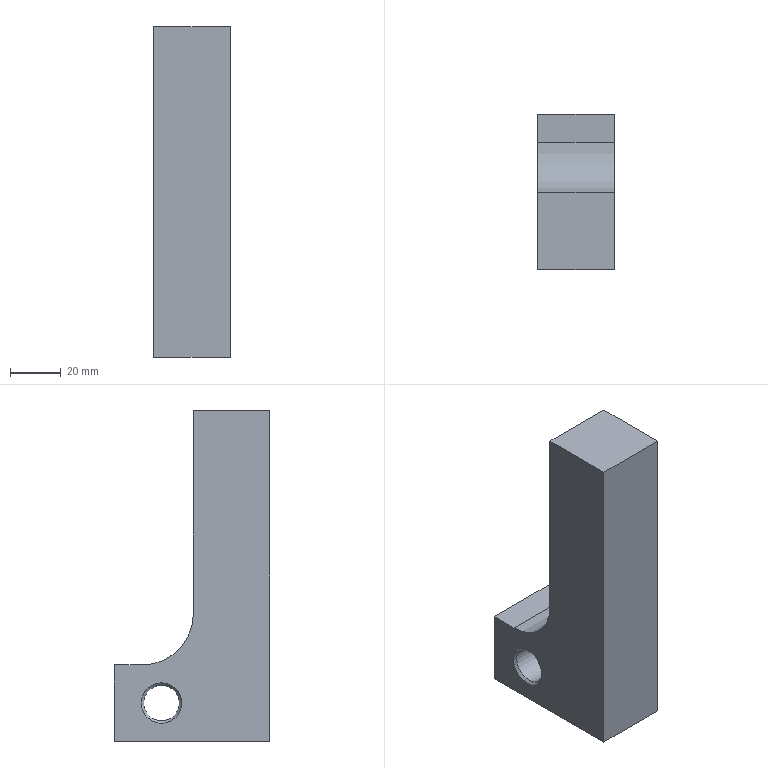Part | STEP file | Tube feed_id550_x_t | 1 solid | 12 faces | box 30 x 61 x 130 mm | volume 142811 mm3 | plane 8 | cylinder 2 | cone 2 | commonest cylinder face diameters 14 x1 40 x1
STEP:
#1=CARTESIAN_POINT('',(0.,0.,0.));
#2=DIRECTION('',(0.,0.,1.));
#3=DIRECTION('',(1.,0.,0.));
#4=AXIS2_PLACEMENT_3D('',#1,#2,#3);
#5=CARTESIAN_POINT('',(176.,541.936,-131.5));
#6=VERTEX_POINT('',#5);
#7=CARTESIAN_POINT('',(176.,552.936,-131.5));
#8=VERTEX_POINT('',#7);
#9=CARTESIAN_POINT('',(176.,521.936,-131.5));
#10=DIRECTION('',(0.,1.,0.));
#11=VECTOR('',#10,1.);
#12=LINE('',#9,#11);
#13=CARTESIAN_POINT('',(176.,521.936,-131.5));
#14=DIRECTION('',(0.,0.,1.));
#15=DIRECTION('',(1.,0.,0.));
#16=AXIS2_PLACEMENT_3D('',#13,#14,#15);
#17=PLANE('',#16);
#18=CARTESIAN_POINT('',(0.,0.));
#19=DIRECTION('',(0.,1.));
#20=VECTOR('',#19,1.);
#21=LINE('',#18,#20);
#22=(GEOMETRIC_REPRESENTATION_CONTEXT(2)PARAMETRIC_REPRESENTATION_CONTEXT()REPRESENTATION_CONTEXT('',''));
#23=DEFINITIONAL_REPRESENTATION('',(#21),#22);
#24=PCURVE('',#17,#23);
#25=CARTESIAN_POINT('',(176.,521.936,-131.5));
#26=DIRECTION('',(1.,0.,0.));
#27=DIRECTION('',(0.,0.,-1.));
#28=AXIS2_PLACEMENT_3D('',#25,#26,#27);
#29=PLANE('',#28);
#30=CARTESIAN_POINT('',(0.,0.));
#31=DIRECTION('',(0.,1.));
#32=VECTOR('',#31,1.);
#33=LINE('',#30,#32);
#34=(GEOMETRIC_REPRESENTATION_CONTEXT(2)PARAMETRIC_REPRESENTATION_CONTEXT()REPRESENTATION_CONTEXT('',''));
#35=DEFINITIONAL_REPRESENTATION('',(#33),#34);
#36=PCURVE('',#29,#35);
#37=SURFACE_CURVE('',#12,(#24,#36),.PCURVE_S1.);
#38=EDGE_CURVE('',#6,#8,#37,.T.);
#39=ORIENTED_EDGE('',*,*,#38,.F.);
#40=CARTESIAN_POINT('',(206.,541.936,-131.5));
#41=VERTEX_POINT('',#40);
#42=CARTESIAN_POINT('',(206.,541.936,-131.5));
#43=DIRECTION('',(1.,0.,0.));
#44=VECTOR('',#43,1.);
#45=LINE('',#42,#44);
#46=CARTESIAN_POINT('',(30.,20.));
#47=DIRECTION('',(1.,0.));
#48=VECTOR('',#47,1.);
#49=LINE('',#46,#48);
#50=(GEOMETRIC_REPRESENTATION_CONTEXT(2)PARAMETRIC_REPRESENTATION_CONTEXT()REPRESENTATION_CONTEXT('',''));
#51=DEFINITIONAL_REPRESENTATION('',(#49),#50);
#52=PCURVE('',#17,#51);
#53=CARTESIAN_POINT('',(176.,541.936,-111.5));
#54=DIRECTION('',(1.,0.,0.));
#55=DIRECTION('',(0.,0.,-1.));
#56=AXIS2_PLACEMENT_3D('',#53,#54,#55);
#57=CYLINDRICAL_SURFACE('',#56,20.);
#58=CARTESIAN_POINT('',(6.283,30.));
#59=DIRECTION('',(0.,1.));
#60=VECTOR('',#59,1.);
#61=LINE('',#58,#60);
#62=(GEOMETRIC_REPRESENTATION_CONTEXT(2)PARAMETRIC_REPRESENTATION_CONTEXT()REPRESENTATION_CONTEXT('',''));
#63=DEFINITIONAL_REPRESENTATION('',(#61),#62);
#64=PCURVE('',#57,#63);
#65=SURFACE_CURVE('',#45,(#52,#64),.PCURVE_S1.);
#66=EDGE_CURVE('',#6,#41,#65,.T.);
#67=ORIENTED_EDGE('',*,*,#66,.T.);
#68=CARTESIAN_POINT('',(206.,552.936,-131.5));
#69=VERTEX_POINT('',#68);
#70=CARTESIAN_POINT('',(206.,521.936,-131.5));
#71=DIRECTION('',(0.,1.,0.));
#72=VECTOR('',#71,1.);
#73=LINE('',#70,#72);
#74=CARTESIAN_POINT('',(30.,0.));
#75=DIRECTION('',(0.,1.));
#76=VECTOR('',#75,1.);
#77=LINE('',#74,#76);
#78=(GEOMETRIC_REPRESENTATION_CONTEXT(2)PARAMETRIC_REPRESENTATION_CONTEXT()REPRESENTATION_CONTEXT('',''));
#79=DEFINITIONAL_REPRESENTATION('',(#77),#78);
#80=PCURVE('',#17,#79);
#81=CARTESIAN_POINT('',(206.,521.936,-131.5));
#82=DIRECTION('',(1.,0.,0.));
#83=DIRECTION('',(0.,0.,-1.));
#84=AXIS2_PLACEMENT_3D('',#81,#82,#83);
#85=PLANE('',#84);
#86=CARTESIAN_POINT('',(0.,0.));
#87=DIRECTION('',(0.,1.));
#88=VECTOR('',#87,1.);
#89=LINE('',#86,#88);
#90=(GEOMETRIC_REPRESENTATION_CONTEXT(2)PARAMETRIC_REPRESENTATION_CONTEXT()REPRESENTATION_CONTEXT('',''));
#91=DEFINITIONAL_REPRESENTATION('',(#89),#90);
#92=PCURVE('',#85,#91);
#93=SURFACE_CURVE('',#73,(#80,#92),.PCURVE_S1.);
#94=EDGE_CURVE('',#41,#69,#93,.T.);
#95=ORIENTED_EDGE('',*,*,#94,.T.);
#96=CARTESIAN_POINT('',(176.,552.936,-131.5));
#97=DIRECTION('',(1.,0.,0.));
#98=VECTOR('',#97,1.);
#99=LINE('',#96,#98);
#100=CARTESIAN_POINT('',(0.,31.));
#101=DIRECTION('',(1.,0.));
#102=VECTOR('',#101,1.);
#103=LINE('',#100,#102);
#104=(GEOMETRIC_REPRESENTATION_CONTEXT(2)PARAMETRIC_REPRESENTATION_CONTEXT()REPRESENTATION_CONTEXT('',''));
#105=DEFINITIONAL_REPRESENTATION('',(#103),#104);
#106=PCURVE('',#17,#105);
#107=CARTESIAN_POINT('',(176.,552.936,-131.5));
#108=DIRECTION('',(0.,1.,0.));
#109=DIRECTION('',(0.,0.,1.));
#110=AXIS2_PLACEMENT_3D('',#107,#108,#109);
#111=PLANE('',#110);
#112=CARTESIAN_POINT('',(0.,0.));
#113=DIRECTION('',(0.,1.));
#114=VECTOR('',#113,1.);
#115=LINE('',#112,#114);
#116=(GEOMETRIC_REPRESENTATION_CONTEXT(2)PARAMETRIC_REPRESENTATION_CONTEXT()REPRESENTATION_CONTEXT('',''));
#117=DEFINITIONAL_REPRESENTATION('',(#115),#116);
#118=PCURVE('',#111,#117);
#119=SURFACE_CURVE('',#99,(#106,#118),.PCURVE_S1.);
#120=EDGE_CURVE('',#8,#69,#119,.T.);
#121=ORIENTED_EDGE('',*,*,#120,.F.);
#122=EDGE_LOOP('',(#39,#67,#95,#121));
#123=FACE_BOUND('',#122,.T.);
#124=ADVANCED_FACE('',(#123),#17,.T.);
#125=CARTESIAN_POINT('',(176.,534.436,-154.5));
#126=VERTEX_POINT('',#125);
#127=CARTESIAN_POINT('',(176.,534.436,-146.5));
#128=DIRECTION('',(1.,0.,0.));
#129=DIRECTION('',(0.,0.,-1.));
#130=AXIS2_PLACEMENT_3D('',#127,#128,#129);
#131=CIRCLE('',#130,8.);
#132=CARTESIAN_POINT('',(15.,12.5));
#133=DIRECTION('',(1.,0.));
#134=AXIS2_PLACEMENT_2D('',#132,#133);
#135=CIRCLE('',#134,8.);
#136=(GEOMETRIC_REPRESENTATION_CONTEXT(2)PARAMETRIC_REPRESENTATION_CONTEXT()REPRESENTATION_CONTEXT('',''));
#137=DEFINITIONAL_REPRESENTATION('',(#135),#136);
#138=PCURVE('',#29,#137);
#139=CARTESIAN_POINT('',(176.,534.436,-146.5));
#140=DIRECTION('',(-1.,0.,0.));
#141=DIRECTION('',(0.,0.,1.));
#142=AXIS2_PLACEMENT_3D('',#139,#140,#141);
#143=CONICAL_SURFACE('',#142,8.,0.7854);
#144=CARTESIAN_POINT('',(9.425,0.));
#145=DIRECTION('',(-1.,0.));
#146=VECTOR('',#145,1.);
#147=LINE('',#144,#146);
#148=(GEOMETRIC_REPRESENTATION_CONTEXT(2)PARAMETRIC_REPRESENTATION_CONTEXT()REPRESENTATION_CONTEXT('',''));
#149=DEFINITIONAL_REPRESENTATION('',(#147),#148);
#150=PCURVE('',#143,#149);
#151=SURFACE_CURVE('',#131,(#138,#150),.PCURVE_S1.);
#152=EDGE_CURVE('',#126,#126,#151,.T.);
#153=ORIENTED_EDGE('',*,*,#152,.T.);
#154=EDGE_LOOP('',(#153));
#155=FACE_BOUND('',#154,.T.);
#156=CARTESIAN_POINT('',(176.,521.936,-31.5));
#157=VERTEX_POINT('',#156);
#158=CARTESIAN_POINT('',(176.,521.936,-111.5));
#159=VERTEX_POINT('',#158);
#160=CARTESIAN_POINT('',(176.,521.936,-31.5));
#161=DIRECTION('',(0.,0.,-1.));
#162=VECTOR('',#161,1.);
#163=LINE('',#160,#162);
#164=CARTESIAN_POINT('',(-100.,0.));
#165=DIRECTION('',(1.,0.));
#166=VECTOR('',#165,1.);
#167=LINE('',#164,#166);
#168=(GEOMETRIC_REPRESENTATION_CONTEXT(2)PARAMETRIC_REPRESENTATION_CONTEXT()REPRESENTATION_CONTEXT('',''));
#169=DEFINITIONAL_REPRESENTATION('',(#167),#168);
#170=PCURVE('',#29,#169);
#171=CARTESIAN_POINT('',(0.,521.936,0.));
#172=DIRECTION('',(0.,-1.,0.));
#173=DIRECTION('',(0.,0.,-1.));
#174=AXIS2_PLACEMENT_3D('',#171,#172,#173);
#175=PLANE('',#174);
#176=CARTESIAN_POINT('',(31.5,176.));
#177=DIRECTION('',(1.,0.));
#178=VECTOR('',#177,1.);
#179=LINE('',#176,#178);
#180=(GEOMETRIC_REPRESENTATION_CONTEXT(2)PARAMETRIC_REPRESENTATION_CONTEXT()REPRESENTATION_CONTEXT('',''));
#181=DEFINITIONAL_REPRESENTATION('',(#179),#180);
#182=PCURVE('',#175,#181);
#183=SURFACE_CURVE('',#163,(#170,#182),.PCURVE_S1.);
#184=EDGE_CURVE('',#157,#159,#183,.T.);
#185=ORIENTED_EDGE('',*,*,#184,.T.);
#186=CARTESIAN_POINT('',(176.,541.936,-111.5));
#187=DIRECTION('',(1.,0.,0.));
#188=DIRECTION('',(0.,0.,-1.));
#189=AXIS2_PLACEMENT_3D('',#186,#187,#188);
#190=CIRCLE('',#189,20.);
#191=CARTESIAN_POINT('',(-20.,20.));
#192=DIRECTION('',(1.,0.));
#193=AXIS2_PLACEMENT_2D('',#191,#192);
#194=CIRCLE('',#193,20.);
#195=(GEOMETRIC_REPRESENTATION_CONTEXT(2)PARAMETRIC_REPRESENTATION_CONTEXT()REPRESENTATION_CONTEXT('',''));
#196=DEFINITIONAL_REPRESENTATION('',(#194),#195);
#197=PCURVE('',#29,#196);
#198=CARTESIAN_POINT('',(0.,0.));
#199=DIRECTION('',(1.,0.));
#200=VECTOR('',#199,1.);
#201=LINE('',#198,#200);
#202=(GEOMETRIC_REPRESENTATION_CONTEXT(2)PARAMETRIC_REPRESENTATION_CONTEXT()REPRESENTATION_CONTEXT('',''));
#203=DEFINITIONAL_REPRESENTATION('',(#201),#202);
#204=PCURVE('',#57,#203);
#205=SURFACE_CURVE('',#190,(#197,#204),.PCURVE_S1.);
#206=EDGE_CURVE('',#159,#6,#205,.T.);
#207=ORIENTED_EDGE('',*,*,#206,.T.);
#208=ORIENTED_EDGE('',*,*,#38,.T.);
#209=CARTESIAN_POINT('',(176.,552.936,-161.5));
#210=VERTEX_POINT('',#209);
#211=CARTESIAN_POINT('',(176.,552.936,-131.5));
#212=DIRECTION('',(0.,0.,-1.));
#213=VECTOR('',#212,1.);
#214=LINE('',#211,#213);
#215=CARTESIAN_POINT('',(0.,31.));
#216=DIRECTION('',(1.,0.));
#217=VECTOR('',#216,1.);
#218=LINE('',#215,#217);
#219=(GEOMETRIC_REPRESENTATION_CONTEXT(2)PARAMETRIC_REPRESENTATION_CONTEXT()REPRESENTATION_CONTEXT('',''));
#220=DEFINITIONAL_REPRESENTATION('',(#218),#219);
#221=PCURVE('',#29,#220);
#222=CARTESIAN_POINT('',(0.,0.));
#223=DIRECTION('',(-1.,0.));
#224=VECTOR('',#223,1.);
#225=LINE('',#222,#224);
#226=(GEOMETRIC_REPRESENTATION_CONTEXT(2)PARAMETRIC_REPRESENTATION_CONTEXT()REPRESENTATION_CONTEXT('',''));
#227=DEFINITIONAL_REPRESENTATION('',(#225),#226);
#228=PCURVE('',#111,#227);
#229=SURFACE_CURVE('',#214,(#221,#228),.PCURVE_S1.);
#230=EDGE_CURVE('',#8,#210,#229,.T.);
#231=ORIENTED_EDGE('',*,*,#230,.T.);
#232=CARTESIAN_POINT('',(176.,491.936,-161.5));
#233=VERTEX_POINT('',#232);
#234=CARTESIAN_POINT('',(176.,521.936,-161.5));
#235=DIRECTION('',(0.,-1.,0.));
#236=VECTOR('',#235,1.);
#237=LINE('',#234,#236);
#238=CARTESIAN_POINT('',(30.,0.));
#239=DIRECTION('',(0.,-1.));
#240=VECTOR('',#239,1.);
#241=LINE('',#238,#240);
#242=(GEOMETRIC_REPRESENTATION_CONTEXT(2)PARAMETRIC_REPRESENTATION_CONTEXT()REPRESENTATION_CONTEXT('',''));
#243=DEFINITIONAL_REPRESENTATION('',(#241),#242);
#244=PCURVE('',#29,#243);
#245=CARTESIAN_POINT('',(176.,521.936,-161.5));
#246=DIRECTION('',(0.,0.,1.));
#247=DIRECTION('',(1.,0.,0.));
#248=AXIS2_PLACEMENT_3D('',#245,#246,#247);
#249=PLANE('',#248);
#250=CARTESIAN_POINT('',(0.,0.));
#251=DIRECTION('',(0.,-1.));
#252=VECTOR('',#251,1.);
#253=LINE('',#250,#252);
#254=(GEOMETRIC_REPRESENTATION_CONTEXT(2)PARAMETRIC_REPRESENTATION_CONTEXT()REPRESENTATION_CONTEXT('',''));
#255=DEFINITIONAL_REPRESENTATION('',(#253),#254);
#256=PCURVE('',#249,#255);
#257=SURFACE_CURVE('',#237,(#244,#256),.PCURVE_S1.);
#258=EDGE_CURVE('',#210,#233,#257,.T.);
#259=ORIENTED_EDGE('',*,*,#258,.T.);
#260=CARTESIAN_POINT('',(176.,491.936,-31.5));
#261=VERTEX_POINT('',#260);
#262=CARTESIAN_POINT('',(176.,491.936,-31.5));
#263=DIRECTION('',(0.,0.,-1.));
#264=VECTOR('',#263,1.);
#265=LINE('',#262,#264);
#266=CARTESIAN_POINT('',(-100.,-30.));
#267=DIRECTION('',(1.,0.));
#268=VECTOR('',#267,1.);
#269=LINE('',#266,#268);
#270=(GEOMETRIC_REPRESENTATION_CONTEXT(2)PARAMETRIC_REPRESENTATION_CONTEXT()REPRESENTATION_CONTEXT('',''));
#271=DEFINITIONAL_REPRESENTATION('',(#269),#270);
#272=PCURVE('',#29,#271);
#273=CARTESIAN_POINT('',(0.,491.936,0.));
#274=DIRECTION('',(0.,-1.,0.));
#275=DIRECTION('',(0.,0.,-1.));
#276=AXIS2_PLACEMENT_3D('',#273,#274,#275);
#277=PLANE('',#276);
#278=CARTESIAN_POINT('',(31.5,176.));
#279=DIRECTION('',(1.,0.));
#280=VECTOR('',#279,1.);
#281=LINE('',#278,#280);
#282=(GEOMETRIC_REPRESENTATION_CONTEXT(2)PARAMETRIC_REPRESENTATION_CONTEXT()REPRESENTATION_CONTEXT('',''));
#283=DEFINITIONAL_REPRESENTATION('',(#281),#282);
#284=PCURVE('',#277,#283);
#285=SURFACE_CURVE('',#265,(#272,#284),.PCURVE_S1.);
#286=EDGE_CURVE('',#261,#233,#285,.T.);
#287=ORIENTED_EDGE('',*,*,#286,.F.);
#288=CARTESIAN_POINT('',(176.,521.936,-31.5));
#289=DIRECTION('',(0.,-1.,0.));
#290=VECTOR('',#289,1.);
#291=LINE('',#288,#290);
#292=CARTESIAN_POINT('',(-100.,0.));
#293=DIRECTION('',(0.,-1.));
#294=VECTOR('',#293,1.);
#295=LINE('',#292,#294);
#296=(GEOMETRIC_REPRESENTATION_CONTEXT(2)PARAMETRIC_REPRESENTATION_CONTEXT()REPRESENTATION_CONTEXT('',''));
#297=DEFINITIONAL_REPRESENTATION('',(#295),#296);
#298=PCURVE('',#29,#297);
#299=CARTESIAN_POINT('',(206.,521.936,-31.5));
#300=DIRECTION('',(0.,0.,1.));
#301=DIRECTION('',(1.,0.,0.));
#302=AXIS2_PLACEMENT_3D('',#299,#300,#301);
#303=PLANE('',#302);
#304=CARTESIAN_POINT('',(-30.,0.));
#305=DIRECTION('',(0.,-1.));
#306=VECTOR('',#305,1.);
#307=LINE('',#304,#306);
#308=(GEOMETRIC_REPRESENTATION_CONTEXT(2)PARAMETRIC_REPRESENTATION_CONTEXT()REPRESENTATION_CONTEXT('',''));
#309=DEFINITIONAL_REPRESENTATION('',(#307),#308);
#310=PCURVE('',#303,#309);
#311=SURFACE_CURVE('',#291,(#298,#310),.PCURVE_S1.);
#312=EDGE_CURVE('',#157,#261,#311,.T.);
#313=ORIENTED_EDGE('',*,*,#312,.F.);
#314=EDGE_LOOP('',(#185,#207,#208,#231,#259,#287,#313));
#315=FACE_BOUND('',#314,.T.);
#316=ADVANCED_FACE('',(#155,#315),#29,.F.);
#317=ORIENTED_EDGE('',*,*,#258,.F.);
#318=CARTESIAN_POINT('',(206.,552.936,-161.5));
#319=VERTEX_POINT('',#318);
#320=CARTESIAN_POINT('',(176.,552.936,-161.5));
#321=DIRECTION('',(1.,0.,0.));
#322=VECTOR('',#321,1.);
#323=LINE('',#320,#322);
#324=CARTESIAN_POINT('',(0.,31.));
#325=DIRECTION('',(1.,0.));
#326=VECTOR('',#325,1.);
#327=LINE('',#324,#326);
#328=(GEOMETRIC_REPRESENTATION_CONTEXT(2)PARAMETRIC_REPRESENTATION_CONTEXT()REPRESENTATION_CONTEXT('',''));
#329=DEFINITIONAL_REPRESENTATION('',(#327),#328);
#330=PCURVE('',#249,#329);
#331=CARTESIAN_POINT('',(-30.,0.));
#332=DIRECTION('',(0.,1.));
#333=VECTOR('',#332,1.);
#334=LINE('',#331,#333);
#335=(GEOMETRIC_REPRESENTATION_CONTEXT(2)PARAMETRIC_REPRESENTATION_CONTEXT()REPRESENTATION_CONTEXT('',''));
#336=DEFINITIONAL_REPRESENTATION('',(#334),#335);
#337=PCURVE('',#111,#336);
#338=SURFACE_CURVE('',#323,(#330,#337),.PCURVE_S1.);
#339=EDGE_CURVE('',#210,#319,#338,.T.);
#340=ORIENTED_EDGE('',*,*,#339,.T.);
#341=CARTESIAN_POINT('',(206.,491.936,-161.5));
#342=VERTEX_POINT('',#341);
#343=CARTESIAN_POINT('',(206.,521.936,-161.5));
#344=DIRECTION('',(0.,-1.,0.));
#345=VECTOR('',#344,1.);
#346=LINE('',#343,#345);
#347=CARTESIAN_POINT('',(30.,0.));
#348=DIRECTION('',(0.,-1.));
#349=VECTOR('',#348,1.);
#350=LINE('',#347,#349);
#351=(GEOMETRIC_REPRESENTATION_CONTEXT(2)PARAMETRIC_REPRESENTATION_CONTEXT()REPRESENTATION_CONTEXT('',''));
#352=DEFINITIONAL_REPRESENTATION('',(#350),#351);
#353=PCURVE('',#249,#352);
#354=CARTESIAN_POINT('',(30.,0.));
#355=DIRECTION('',(0.,-1.));
#356=VECTOR('',#355,1.);
#357=LINE('',#354,#356);
#358=(GEOMETRIC_REPRESENTATION_CONTEXT(2)PARAMETRIC_REPRESENTATION_CONTEXT()REPRESENTATION_CONTEXT('',''));
#359=DEFINITIONAL_REPRESENTATION('',(#357),#358);
#360=PCURVE('',#85,#359);
#361=SURFACE_CURVE('',#346,(#353,#360),.PCURVE_S1.);
#362=EDGE_CURVE('',#319,#342,#361,.T.);
#363=ORIENTED_EDGE('',*,*,#362,.T.);
#364=CARTESIAN_POINT('',(176.,491.936,-161.5));
#365=DIRECTION('',(1.,0.,0.));
#366=VECTOR('',#365,1.);
#367=LINE('',#364,#366);
#368=CARTESIAN_POINT('',(0.,-30.));
#369=DIRECTION('',(1.,0.));
#370=VECTOR('',#369,1.);
#371=LINE('',#368,#370);
#372=(GEOMETRIC_REPRESENTATION_CONTEXT(2)PARAMETRIC_REPRESENTATION_CONTEXT()REPRESENTATION_CONTEXT('',''));
#373=DEFINITIONAL_REPRESENTATION('',(#371),#372);
#374=PCURVE('',#249,#373);
#375=CARTESIAN_POINT('',(161.5,176.));
#376=DIRECTION('',(0.,1.));
#377=VECTOR('',#376,1.);
#378=LINE('',#375,#377);
#379=(GEOMETRIC_REPRESENTATION_CONTEXT(2)PARAMETRIC_REPRESENTATION_CONTEXT()REPRESENTATION_CONTEXT('',''));
#380=DEFINITIONAL_REPRESENTATION('',(#378),#379);
#381=PCURVE('',#277,#380);
#382=SURFACE_CURVE('',#367,(#374,#381),.PCURVE_S1.);
#383=EDGE_CURVE('',#233,#342,#382,.T.);
#384=ORIENTED_EDGE('',*,*,#383,.F.);
#385=EDGE_LOOP('',(#317,#340,#363,#384));
#386=FACE_BOUND('',#385,.T.);
#387=ADVANCED_FACE('',(#386),#249,.F.);
#388=CARTESIAN_POINT('',(206.,534.436,-154.5));
#389=VERTEX_POINT('',#388);
#390=CARTESIAN_POINT('',(206.,534.436,-146.5));
#391=DIRECTION('',(-1.,0.,0.));
#392=DIRECTION('',(0.,0.,-1.));
#393=AXIS2_PLACEMENT_3D('',#390,#391,#392);
#394=CIRCLE('',#393,8.);
#395=CARTESIAN_POINT('',(23.,12.5));
#396=CARTESIAN_POINT('',(23.,-1.356));
#397=CARTESIAN_POINT('',(11.,5.572));
#398=CARTESIAN_POINT('',(-1.,12.5));
#399=CARTESIAN_POINT('',(11.,19.428));
#400=CARTESIAN_POINT('',(23.,26.356));
#401=CARTESIAN_POINT('',(23.,12.5));
#402=(BOUNDED_CURVE()B_SPLINE_CURVE(2,(#395,#396,#397,#398,#399,#400,#401),.UNSPECIFIED.,.T.,.F.)B_SPLINE_CURVE_WITH_KNOTS((1,2,2,2,2,1),(-2.094,0.,2.094,4.189,6.283,8.378),.UNSPECIFIED.)CURVE()GEOMETRIC_REPRESENTATION_ITEM()RATIONAL_B_SPLINE_CURVE((1.,0.5,1.,0.5,1.,0.5,1.))REPRESENTATION_ITEM(''));
#403=(GEOMETRIC_REPRESENTATION_CONTEXT(2)PARAMETRIC_REPRESENTATION_CONTEXT()REPRESENTATION_CONTEXT('',''));
#404=DEFINITIONAL_REPRESENTATION('',(#402),#403);
#405=PCURVE('',#85,#404);
#406=CARTESIAN_POINT('',(206.,534.436,-146.5));
#407=DIRECTION('',(1.,0.,0.));
#408=DIRECTION('',(0.,0.,-1.));
#409=AXIS2_PLACEMENT_3D('',#406,#407,#408);
#410=CONICAL_SURFACE('',#409,8.,0.7854);
#411=CARTESIAN_POINT('',(6.283,0.));
#412=DIRECTION('',(-1.,0.));
#413=VECTOR('',#412,1.);
#414=LINE('',#411,#413);
#415=(GEOMETRIC_REPRESENTATION_CONTEXT(2)PARAMETRIC_REPRESENTATION_CONTEXT()REPRESENTATION_CONTEXT('',''));
#416=DEFINITIONAL_REPRESENTATION('',(#414),#415);
#417=PCURVE('',#410,#416);
#418=SURFACE_CURVE('',#394,(#405,#417),.PCURVE_S1.);
#419=EDGE_CURVE('',#389,#389,#418,.T.);
#420=ORIENTED_EDGE('',*,*,#419,.T.);
#421=EDGE_LOOP('',(#420));
#422=FACE_BOUND('',#421,.T.);
#423=ORIENTED_EDGE('',*,*,#94,.F.);
#424=CARTESIAN_POINT('',(206.,521.936,-111.5));
#425=VERTEX_POINT('',#424);
#426=CARTESIAN_POINT('',(206.,541.936,-111.5));
#427=DIRECTION('',(-1.,0.,0.));
#428=DIRECTION('',(0.,0.,-1.));
#429=AXIS2_PLACEMENT_3D('',#426,#427,#428);
#430=CIRCLE('',#429,20.);
#431=CARTESIAN_POINT('',(0.,20.));
#432=CARTESIAN_POINT('',(0.,-14.641));
#433=CARTESIAN_POINT('',(-30.,2.679));
#434=CARTESIAN_POINT('',(-60.,20.));
#435=CARTESIAN_POINT('',(-30.,37.321));
#436=CARTESIAN_POINT('',(0.,54.641));
#437=CARTESIAN_POINT('',(0.,20.));
#438=(BOUNDED_CURVE()B_SPLINE_CURVE(2,(#431,#432,#433,#434,#435,#436,#437),.UNSPECIFIED.,.T.,.F.)B_SPLINE_CURVE_WITH_KNOTS((1,2,2,2,2,1),(-2.094,0.,2.094,4.189,6.283,8.378),.UNSPECIFIED.)CURVE()GEOMETRIC_REPRESENTATION_ITEM()RATIONAL_B_SPLINE_CURVE((1.,0.5,1.,0.5,1.,0.5,1.))REPRESENTATION_ITEM(''));
#439=(GEOMETRIC_REPRESENTATION_CONTEXT(2)PARAMETRIC_REPRESENTATION_CONTEXT()REPRESENTATION_CONTEXT('',''));
#440=DEFINITIONAL_REPRESENTATION('',(#438),#439);
#441=PCURVE('',#85,#440);
#442=CARTESIAN_POINT('',(6.283,30.));
#443=DIRECTION('',(-1.,0.));
#444=VECTOR('',#443,1.);
#445=LINE('',#442,#444);
#446=(GEOMETRIC_REPRESENTATION_CONTEXT(2)PARAMETRIC_REPRESENTATION_CONTEXT()REPRESENTATION_CONTEXT('',''));
#447=DEFINITIONAL_REPRESENTATION('',(#445),#446);
#448=PCURVE('',#57,#447);
#449=SURFACE_CURVE('',#430,(#441,#448),.PCURVE_S1.);
#450=EDGE_CURVE('',#41,#425,#449,.T.);
#451=ORIENTED_EDGE('',*,*,#450,.T.);
#452=CARTESIAN_POINT('',(206.,521.936,-31.5));
#453=VERTEX_POINT('',#452);
#454=CARTESIAN_POINT('',(206.,521.936,-161.5));
#455=DIRECTION('',(0.,0.,1.));
#456=VECTOR('',#455,1.);
#457=LINE('',#454,#456);
#458=CARTESIAN_POINT('',(30.,0.));
#459=DIRECTION('',(-1.,0.));
#460=VECTOR('',#459,1.);
#461=LINE('',#458,#460);
#462=(GEOMETRIC_REPRESENTATION_CONTEXT(2)PARAMETRIC_REPRESENTATION_CONTEXT()REPRESENTATION_CONTEXT('',''));
#463=DEFINITIONAL_REPRESENTATION('',(#461),#462);
#464=PCURVE('',#85,#463);
#465=CARTESIAN_POINT('',(161.5,206.));
#466=DIRECTION('',(-1.,0.));
#467=VECTOR('',#466,1.);
#468=LINE('',#465,#467);
#469=(GEOMETRIC_REPRESENTATION_CONTEXT(2)PARAMETRIC_REPRESENTATION_CONTEXT()REPRESENTATION_CONTEXT('',''));
#470=DEFINITIONAL_REPRESENTATION('',(#468),#469);
#471=PCURVE('',#175,#470);
#472=SURFACE_CURVE('',#457,(#464,#471),.PCURVE_S1.);
#473=EDGE_CURVE('',#425,#453,#472,.T.);
#474=ORIENTED_EDGE('',*,*,#473,.T.);
#475=CARTESIAN_POINT('',(206.,491.936,-31.5));
#476=VERTEX_POINT('',#475);
#477=CARTESIAN_POINT('',(206.,521.936,-31.5));
#478=DIRECTION('',(0.,-1.,0.));
#479=VECTOR('',#478,1.);
#480=LINE('',#477,#479);
#481=CARTESIAN_POINT('',(-100.,0.));
#482=DIRECTION('',(0.,-1.));
#483=VECTOR('',#482,1.);
#484=LINE('',#481,#483);
#485=(GEOMETRIC_REPRESENTATION_CONTEXT(2)PARAMETRIC_REPRESENTATION_CONTEXT()REPRESENTATION_CONTEXT('',''));
#486=DEFINITIONAL_REPRESENTATION('',(#484),#485);
#487=PCURVE('',#85,#486);
#488=CARTESIAN_POINT('',(0.,0.));
#489=DIRECTION('',(0.,-1.));
#490=VECTOR('',#489,1.);
#491=LINE('',#488,#490);
#492=(GEOMETRIC_REPRESENTATION_CONTEXT(2)PARAMETRIC_REPRESENTATION_CONTEXT()REPRESENTATION_CONTEXT('',''));
#493=DEFINITIONAL_REPRESENTATION('',(#491),#492);
#494=PCURVE('',#303,#493);
#495=SURFACE_CURVE('',#480,(#487,#494),.PCURVE_S1.);
#496=EDGE_CURVE('',#453,#476,#495,.T.);
#497=ORIENTED_EDGE('',*,*,#496,.T.);
#498=CARTESIAN_POINT('',(206.,491.936,-161.5));
#499=DIRECTION('',(0.,0.,1.));
#500=VECTOR('',#499,1.);
#501=LINE('',#498,#500);
#502=CARTESIAN_POINT('',(30.,-30.));
#503=DIRECTION('',(-1.,0.));
#504=VECTOR('',#503,1.);
#505=LINE('',#502,#504);
#506=(GEOMETRIC_REPRESENTATION_CONTEXT(2)PARAMETRIC_REPRESENTATION_CONTEXT()REPRESENTATION_CONTEXT('',''));
#507=DEFINITIONAL_REPRESENTATION('',(#505),#506);
#508=PCURVE('',#85,#507);
#509=CARTESIAN_POINT('',(161.5,206.));
#510=DIRECTION('',(-1.,0.));
#511=VECTOR('',#510,1.);
#512=LINE('',#509,#511);
#513=(GEOMETRIC_REPRESENTATION_CONTEXT(2)PARAMETRIC_REPRESENTATION_CONTEXT()REPRESENTATION_CONTEXT('',''));
#514=DEFINITIONAL_REPRESENTATION('',(#512),#513);
#515=PCURVE('',#277,#514);
#516=SURFACE_CURVE('',#501,(#508,#515),.PCURVE_S1.);
#517=EDGE_CURVE('',#342,#476,#516,.T.);
#518=ORIENTED_EDGE('',*,*,#517,.F.);
#519=ORIENTED_EDGE('',*,*,#362,.F.);
#520=CARTESIAN_POINT('',(206.,552.936,-131.5));
#521=DIRECTION('',(0.,0.,-1.));
#522=VECTOR('',#521,1.);
#523=LINE('',#520,#522);
#524=CARTESIAN_POINT('',(0.,31.));
#525=DIRECTION('',(1.,0.));
#526=VECTOR('',#525,1.);
#527=LINE('',#524,#526);
#528=(GEOMETRIC_REPRESENTATION_CONTEXT(2)PARAMETRIC_REPRESENTATION_CONTEXT()REPRESENTATION_CONTEXT('',''));
#529=DEFINITIONAL_REPRESENTATION('',(#527),#528);
#530=PCURVE('',#85,#529);
#531=CARTESIAN_POINT('',(0.,30.));
#532=DIRECTION('',(-1.,0.));
#533=VECTOR('',#532,1.);
#534=LINE('',#531,#533);
#535=(GEOMETRIC_REPRESENTATION_CONTEXT(2)PARAMETRIC_REPRESENTATION_CONTEXT()REPRESENTATION_CONTEXT('',''));
#536=DEFINITIONAL_REPRESENTATION('',(#534),#535);
#537=PCURVE('',#111,#536);
#538=SURFACE_CURVE('',#523,(#530,#537),.PCURVE_S1.);
#539=EDGE_CURVE('',#69,#319,#538,.T.);
#540=ORIENTED_EDGE('',*,*,#539,.F.);
#541=EDGE_LOOP('',(#423,#451,#474,#497,#518,#519,#540));
#542=FACE_BOUND('',#541,.T.);
#543=ADVANCED_FACE('',(#422,#542),#85,.T.);
#544=ORIENTED_EDGE('',*,*,#339,.F.);
#545=ORIENTED_EDGE('',*,*,#230,.F.);
#546=ORIENTED_EDGE('',*,*,#120,.T.);
#547=ORIENTED_EDGE('',*,*,#539,.T.);
#548=EDGE_LOOP('',(#544,#545,#546,#547));
#549=FACE_BOUND('',#548,.T.);
#550=ADVANCED_FACE('',(#549),#111,.T.);
#551=CARTESIAN_POINT('',(206.,491.936,-31.5));
#552=DIRECTION('',(-1.,0.,0.));
#553=VECTOR('',#552,1.);
#554=LINE('',#551,#553);
#555=CARTESIAN_POINT('',(0.,-30.));
#556=DIRECTION('',(-1.,0.));
#557=VECTOR('',#556,1.);
#558=LINE('',#555,#557);
#559=(GEOMETRIC_REPRESENTATION_CONTEXT(2)PARAMETRIC_REPRESENTATION_CONTEXT()REPRESENTATION_CONTEXT('',''));
#560=DEFINITIONAL_REPRESENTATION('',(#558),#559);
#561=PCURVE('',#303,#560);
#562=CARTESIAN_POINT('',(31.5,206.));
#563=DIRECTION('',(0.,-1.));
#564=VECTOR('',#563,1.);
#565=LINE('',#562,#564);
#566=(GEOMETRIC_REPRESENTATION_CONTEXT(2)PARAMETRIC_REPRESENTATION_CONTEXT()REPRESENTATION_CONTEXT('',''));
#567=DEFINITIONAL_REPRESENTATION('',(#565),#566);
#568=PCURVE('',#277,#567);
#569=SURFACE_CURVE('',#554,(#561,#568),.PCURVE_S1.);
#570=EDGE_CURVE('',#476,#261,#569,.T.);
#571=ORIENTED_EDGE('',*,*,#570,.F.);
#572=ORIENTED_EDGE('',*,*,#496,.F.);
#573=CARTESIAN_POINT('',(206.,521.936,-31.5));
#574=DIRECTION('',(-1.,0.,0.));
#575=VECTOR('',#574,1.);
#576=LINE('',#573,#575);
#577=CARTESIAN_POINT('',(0.,0.));
#578=DIRECTION('',(-1.,0.));
#579=VECTOR('',#578,1.);
#580=LINE('',#577,#579);
#581=(GEOMETRIC_REPRESENTATION_CONTEXT(2)PARAMETRIC_REPRESENTATION_CONTEXT()REPRESENTATION_CONTEXT('',''));
#582=DEFINITIONAL_REPRESENTATION('',(#580),#581);
#583=PCURVE('',#303,#582);
#584=CARTESIAN_POINT('',(31.5,206.));
#585=DIRECTION('',(0.,-1.));
#586=VECTOR('',#585,1.);
#587=LINE('',#584,#586);
#588=(GEOMETRIC_REPRESENTATION_CONTEXT(2)PARAMETRIC_REPRESENTATION_CONTEXT()REPRESENTATION_CONTEXT('',''));
#589=DEFINITIONAL_REPRESENTATION('',(#587),#588);
#590=PCURVE('',#175,#589);
#591=SURFACE_CURVE('',#576,(#583,#590),.PCURVE_S1.);
#592=EDGE_CURVE('',#453,#157,#591,.T.);
#593=ORIENTED_EDGE('',*,*,#592,.T.);
#594=ORIENTED_EDGE('',*,*,#312,.T.);
#595=EDGE_LOOP('',(#571,#572,#593,#594));
#596=FACE_BOUND('',#595,.T.);
#597=ADVANCED_FACE('',(#596),#303,.T.);
#598=ORIENTED_EDGE('',*,*,#473,.F.);
#599=CARTESIAN_POINT('',(176.,521.936,-111.5));
#600=DIRECTION('',(-1.,0.,0.));
#601=VECTOR('',#600,1.);
#602=LINE('',#599,#601);
#603=CARTESIAN_POINT('',(111.5,176.));
#604=DIRECTION('',(0.,-1.));
#605=VECTOR('',#604,1.);
#606=LINE('',#603,#605);
#607=(GEOMETRIC_REPRESENTATION_CONTEXT(2)PARAMETRIC_REPRESENTATION_CONTEXT()REPRESENTATION_CONTEXT('',''));
#608=DEFINITIONAL_REPRESENTATION('',(#606),#607);
#609=PCURVE('',#175,#608);
#610=CARTESIAN_POINT('',(4.712,0.));
#611=DIRECTION('',(0.,-1.));
#612=VECTOR('',#611,1.);
#613=LINE('',#610,#612);
#614=(GEOMETRIC_REPRESENTATION_CONTEXT(2)PARAMETRIC_REPRESENTATION_CONTEXT()REPRESENTATION_CONTEXT('',''));
#615=DEFINITIONAL_REPRESENTATION('',(#613),#614);
#616=PCURVE('',#57,#615);
#617=SURFACE_CURVE('',#602,(#609,#616),.PCURVE_S1.);
#618=EDGE_CURVE('',#425,#159,#617,.T.);
#619=ORIENTED_EDGE('',*,*,#618,.T.);
#620=ORIENTED_EDGE('',*,*,#184,.F.);
#621=ORIENTED_EDGE('',*,*,#592,.F.);
#622=EDGE_LOOP('',(#598,#619,#620,#621));
#623=FACE_BOUND('',#622,.T.);
#624=ADVANCED_FACE('',(#623),#175,.F.);
#625=ORIENTED_EDGE('',*,*,#286,.T.);
#626=ORIENTED_EDGE('',*,*,#383,.T.);
#627=ORIENTED_EDGE('',*,*,#517,.T.);
#628=ORIENTED_EDGE('',*,*,#570,.T.);
#629=EDGE_LOOP('',(#625,#626,#627,#628));
#630=FACE_BOUND('',#629,.T.);
#631=ADVANCED_FACE('',(#630),#277,.T.);
#632=ORIENTED_EDGE('',*,*,#66,.T.);
#633=ORIENTED_EDGE('',*,*,#450,.T.);
#634=ORIENTED_EDGE('',*,*,#618,.T.);
#635=ORIENTED_EDGE('',*,*,#206,.T.);
#636=EDGE_LOOP('',(#632,#633,#634,#635));
#637=FACE_BOUND('',#636,.F.);
#638=ADVANCED_FACE('',(#637),#57,.F.);
#639=CARTESIAN_POINT('',(177.,534.436,-139.5));
#640=VERTEX_POINT('',#639);
#641=CARTESIAN_POINT('',(177.,534.436,-153.5));
#642=VERTEX_POINT('',#641);
#643=CARTESIAN_POINT('',(177.,534.436,-146.5));
#644=DIRECTION('',(-1.,0.,0.));
#645=DIRECTION('',(0.,0.,-1.));
#646=AXIS2_PLACEMENT_3D('',#643,#644,#645);
#647=CIRCLE('',#646,7.);
#648=CARTESIAN_POINT('',(206.,534.436,-146.5));
#649=DIRECTION('',(-1.,0.,0.));
#650=DIRECTION('',(0.,0.,1.));
#651=AXIS2_PLACEMENT_3D('',#648,#649,#650);
#652=CYLINDRICAL_SURFACE('',#651,7.);
#653=CARTESIAN_POINT('',(-3.142,29.));
#654=DIRECTION('',(1.,0.));
#655=VECTOR('',#654,1.);
#656=LINE('',#653,#655);
#657=(GEOMETRIC_REPRESENTATION_CONTEXT(2)PARAMETRIC_REPRESENTATION_CONTEXT()REPRESENTATION_CONTEXT('',''));
#658=DEFINITIONAL_REPRESENTATION('',(#656),#657);
#659=PCURVE('',#652,#658);
#660=CARTESIAN_POINT('',(3.142,-1.));
#661=DIRECTION('',(1.,0.));
#662=VECTOR('',#661,1.);
#663=LINE('',#660,#662);
#664=(GEOMETRIC_REPRESENTATION_CONTEXT(2)PARAMETRIC_REPRESENTATION_CONTEXT()REPRESENTATION_CONTEXT('',''));
#665=DEFINITIONAL_REPRESENTATION('',(#663),#664);
#666=PCURVE('',#143,#665);
#667=SURFACE_CURVE('',#647,(#659,#666),.PCURVE_S1.);
#668=EDGE_CURVE('',#640,#642,#667,.T.);
#669=ORIENTED_EDGE('',*,*,#668,.F.);
#670=CARTESIAN_POINT('',(205.,534.436,-139.5));
#671=VERTEX_POINT('',#670);
#672=CARTESIAN_POINT('',(205.,534.436,-139.5));
#673=CARTESIAN_POINT('',(177.,534.436,-139.5));
#674=B_SPLINE_CURVE_WITH_KNOTS('',1,(#672,#673),.UNSPECIFIED.,.F.,.F.,(2,2),(1.,29.),.PIECEWISE_BEZIER_KNOTS.);
#675=CARTESIAN_POINT('',(0.,0.));
#676=DIRECTION('',(0.,1.));
#677=VECTOR('',#676,1.);
#678=LINE('',#675,#677);
#679=(GEOMETRIC_REPRESENTATION_CONTEXT(2)PARAMETRIC_REPRESENTATION_CONTEXT()REPRESENTATION_CONTEXT('',''));
#680=DEFINITIONAL_REPRESENTATION('',(#678),#679);
#681=PCURVE('',#652,#680);
#682=CARTESIAN_POINT('',(6.283,0.));
#683=DIRECTION('',(0.,1.));
#684=VECTOR('',#683,1.);
#685=LINE('',#682,#684);
#686=(GEOMETRIC_REPRESENTATION_CONTEXT(2)PARAMETRIC_REPRESENTATION_CONTEXT()REPRESENTATION_CONTEXT('',''));
#687=DEFINITIONAL_REPRESENTATION('',(#685),#686);
#688=PCURVE('',#652,#687);
#689=SEAM_CURVE('',#674,(#681,#688),.PCURVE_S1.);
#690=EDGE_CURVE('',#671,#640,#689,.T.);
#691=ORIENTED_EDGE('',*,*,#690,.F.);
#692=CARTESIAN_POINT('',(205.,534.436,-153.5));
#693=VERTEX_POINT('',#692);
#694=CARTESIAN_POINT('',(205.,534.436,-146.5));
#695=DIRECTION('',(1.,0.,0.));
#696=DIRECTION('',(0.,0.,1.));
#697=AXIS2_PLACEMENT_3D('',#694,#695,#696);
#698=CIRCLE('',#697,7.);
#699=CARTESIAN_POINT('',(6.283,1.));
#700=DIRECTION('',(-1.,0.));
#701=VECTOR('',#700,1.);
#702=LINE('',#699,#701);
#703=(GEOMETRIC_REPRESENTATION_CONTEXT(2)PARAMETRIC_REPRESENTATION_CONTEXT()REPRESENTATION_CONTEXT('',''));
#704=DEFINITIONAL_REPRESENTATION('',(#702),#703);
#705=PCURVE('',#652,#704);
#706=CARTESIAN_POINT('',(-3.142,-1.));
#707=DIRECTION('',(1.,0.));
#708=VECTOR('',#707,1.);
#709=LINE('',#706,#708);
#710=(GEOMETRIC_REPRESENTATION_CONTEXT(2)PARAMETRIC_REPRESENTATION_CONTEXT()REPRESENTATION_CONTEXT('',''));
#711=DEFINITIONAL_REPRESENTATION('',(#709),#710);
#712=PCURVE('',#410,#711);
#713=SURFACE_CURVE('',#698,(#705,#712),.PCURVE_S1.);
#714=EDGE_CURVE('',#693,#671,#713,.T.);
#715=ORIENTED_EDGE('',*,*,#714,.F.);
#716=CARTESIAN_POINT('',(205.,534.436,-146.5));
#717=DIRECTION('',(1.,0.,0.));
#718=DIRECTION('',(0.,0.,1.));
#719=AXIS2_PLACEMENT_3D('',#716,#717,#718);
#720=CIRCLE('',#719,7.);
#721=CARTESIAN_POINT('',(6.283,1.));
#722=DIRECTION('',(-1.,0.));
#723=VECTOR('',#722,1.);
#724=LINE('',#721,#723);
#725=(GEOMETRIC_REPRESENTATION_CONTEXT(2)PARAMETRIC_REPRESENTATION_CONTEXT()REPRESENTATION_CONTEXT('',''));
#726=DEFINITIONAL_REPRESENTATION('',(#724),#725);
#727=PCURVE('',#652,#726);
#728=CARTESIAN_POINT('',(3.142,-1.));
#729=DIRECTION('',(1.,0.));
#730=VECTOR('',#729,1.);
#731=LINE('',#728,#730);
#732=(GEOMETRIC_REPRESENTATION_CONTEXT(2)PARAMETRIC_REPRESENTATION_CONTEXT()REPRESENTATION_CONTEXT('',''));
#733=DEFINITIONAL_REPRESENTATION('',(#731),#732);
#734=PCURVE('',#410,#733);
#735=SURFACE_CURVE('',#720,(#727,#734),.PCURVE_S1.);
#736=EDGE_CURVE('',#671,#693,#735,.T.);
#737=ORIENTED_EDGE('',*,*,#736,.F.);
#738=ORIENTED_EDGE('',*,*,#690,.T.);
#739=CARTESIAN_POINT('',(177.,534.436,-146.5));
#740=DIRECTION('',(-1.,0.,0.));
#741=DIRECTION('',(0.,0.,-1.));
#742=AXIS2_PLACEMENT_3D('',#739,#740,#741);
#743=CIRCLE('',#742,7.);
#744=CARTESIAN_POINT('',(3.142,29.));
#745=DIRECTION('',(1.,0.));
#746=VECTOR('',#745,1.);
#747=LINE('',#744,#746);
#748=(GEOMETRIC_REPRESENTATION_CONTEXT(2)PARAMETRIC_REPRESENTATION_CONTEXT()REPRESENTATION_CONTEXT('',''));
#749=DEFINITIONAL_REPRESENTATION('',(#747),#748);
#750=PCURVE('',#652,#749);
#751=CARTESIAN_POINT('',(3.142,-1.));
#752=DIRECTION('',(1.,0.));
#753=VECTOR('',#752,1.);
#754=LINE('',#751,#753);
#755=(GEOMETRIC_REPRESENTATION_CONTEXT(2)PARAMETRIC_REPRESENTATION_CONTEXT()REPRESENTATION_CONTEXT('',''));
#756=DEFINITIONAL_REPRESENTATION('',(#754),#755);
#757=PCURVE('',#143,#756);
#758=SURFACE_CURVE('',#743,(#750,#757),.PCURVE_S1.);
#759=EDGE_CURVE('',#642,#640,#758,.T.);
#760=ORIENTED_EDGE('',*,*,#759,.F.);
#761=EDGE_LOOP('',(#669,#691,#715,#737,#738,#760));
#762=FACE_BOUND('',#761,.F.);
#763=ADVANCED_FACE('',(#762),#652,.F.);
#764=ORIENTED_EDGE('',*,*,#736,.T.);
#765=CARTESIAN_POINT('',(205.,534.436,-153.5));
#766=CARTESIAN_POINT('',(206.,534.436,-154.5));
#767=B_SPLINE_CURVE_WITH_KNOTS('',1,(#765,#766),.UNSPECIFIED.,.F.,.F.,(2,2),(-1.414,0.),.PIECEWISE_BEZIER_KNOTS.);
#768=CARTESIAN_POINT('',(6.283,0.));
#769=DIRECTION('',(0.,1.));
#770=VECTOR('',#769,1.);
#771=LINE('',#768,#770);
#772=(GEOMETRIC_REPRESENTATION_CONTEXT(2)PARAMETRIC_REPRESENTATION_CONTEXT()REPRESENTATION_CONTEXT('',''));
#773=DEFINITIONAL_REPRESENTATION('',(#771),#772);
#774=PCURVE('',#410,#773);
#775=CARTESIAN_POINT('',(0.,0.));
#776=DIRECTION('',(0.,1.));
#777=VECTOR('',#776,1.);
#778=LINE('',#775,#777);
#779=(GEOMETRIC_REPRESENTATION_CONTEXT(2)PARAMETRIC_REPRESENTATION_CONTEXT()REPRESENTATION_CONTEXT('',''));
#780=DEFINITIONAL_REPRESENTATION('',(#778),#779);
#781=PCURVE('',#410,#780);
#782=SEAM_CURVE('',#767,(#774,#781),.PCURVE_S1.);
#783=EDGE_CURVE('',#693,#389,#782,.T.);
#784=ORIENTED_EDGE('',*,*,#783,.T.);
#785=ORIENTED_EDGE('',*,*,#419,.T.);
#786=ORIENTED_EDGE('',*,*,#783,.F.);
#787=ORIENTED_EDGE('',*,*,#714,.T.);
#788=EDGE_LOOP('',(#764,#784,#785,#786,#787));
#789=FACE_BOUND('',#788,.F.);
#790=ADVANCED_FACE('',(#789),#410,.F.);
#791=ORIENTED_EDGE('',*,*,#668,.T.);
#792=CARTESIAN_POINT('',(177.,534.436,-153.5));
#793=CARTESIAN_POINT('',(176.,534.436,-154.5));
#794=B_SPLINE_CURVE_WITH_KNOTS('',1,(#792,#793),.UNSPECIFIED.,.F.,.F.,(2,2),(-1.414,0.),.PIECEWISE_BEZIER_KNOTS.);
#795=CARTESIAN_POINT('',(9.425,0.));
#796=DIRECTION('',(0.,1.));
#797=VECTOR('',#796,1.);
#798=LINE('',#795,#797);
#799=(GEOMETRIC_REPRESENTATION_CONTEXT(2)PARAMETRIC_REPRESENTATION_CONTEXT()REPRESENTATION_CONTEXT('',''));
#800=DEFINITIONAL_REPRESENTATION('',(#798),#799);
#801=PCURVE('',#143,#800);
#802=CARTESIAN_POINT('',(3.142,0.));
#803=DIRECTION('',(0.,1.));
#804=VECTOR('',#803,1.);
#805=LINE('',#802,#804);
#806=(GEOMETRIC_REPRESENTATION_CONTEXT(2)PARAMETRIC_REPRESENTATION_CONTEXT()REPRESENTATION_CONTEXT('',''));
#807=DEFINITIONAL_REPRESENTATION('',(#805),#806);
#808=PCURVE('',#143,#807);
#809=SEAM_CURVE('',#794,(#801,#808),.PCURVE_S1.);
#810=EDGE_CURVE('',#642,#126,#809,.T.);
#811=ORIENTED_EDGE('',*,*,#810,.T.);
#812=ORIENTED_EDGE('',*,*,#152,.T.);
#813=ORIENTED_EDGE('',*,*,#810,.F.);
#814=ORIENTED_EDGE('',*,*,#759,.T.);
#815=EDGE_LOOP('',(#791,#811,#812,#813,#814));
#816=FACE_BOUND('',#815,.F.);
#817=ADVANCED_FACE('',(#816),#143,.F.);
#818=CLOSED_SHELL('',(#124,#316,#387,#543,#550,#597,#624,#631,#638,#763,#790,#817));
#819=MANIFOLD_SOLID_BREP('',#818);
#820=(LENGTH_UNIT()NAMED_UNIT(*)SI_UNIT(.MILLI.,.METRE.));
#821=UNCERTAINTY_MEASURE_WITH_UNIT(LENGTH_MEASURE(0.000002),#820,'','');
#822=(NAMED_UNIT(*)PLANE_ANGLE_UNIT()SI_UNIT($,.RADIAN.));
#823=(NAMED_UNIT(*)SI_UNIT($,.STERADIAN.)SOLID_ANGLE_UNIT());
#824=(GEOMETRIC_REPRESENTATION_CONTEXT(3)GLOBAL_UNCERTAINTY_ASSIGNED_CONTEXT((#821))GLOBAL_UNIT_ASSIGNED_CONTEXT((#820,#822,#823))REPRESENTATION_CONTEXT('',''));
#825=ADVANCED_BREP_SHAPE_REPRESENTATION('',(#4,#819),#824);